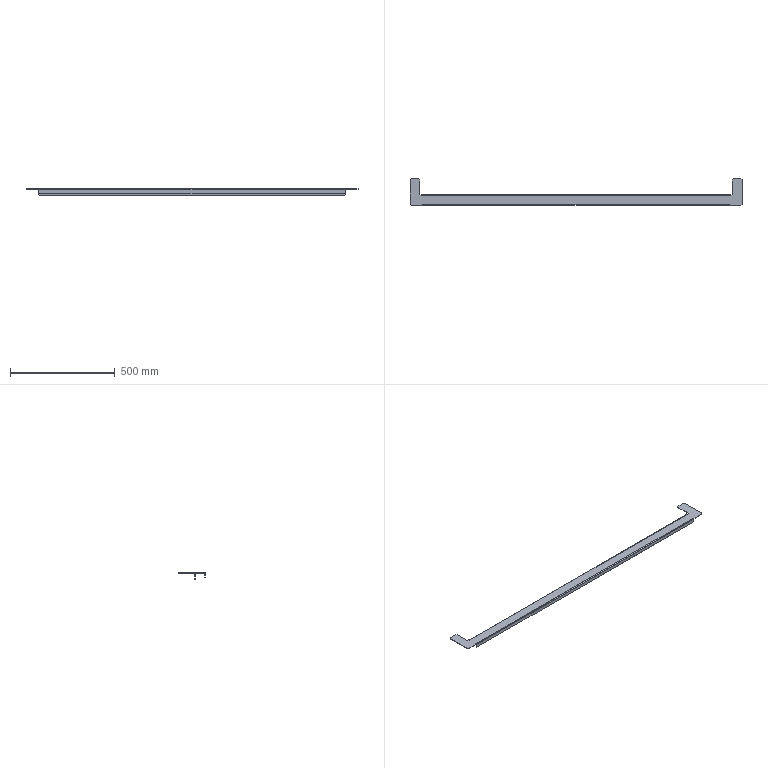Part | STEP file | SYL_0392D6J1SYL0380DJ10-1266534 | 1 solid | 50 faces | box 1586 x 125 x 30 mm | volume 300199 mm3 | plane 46 | cylinder 4 | commonest cylinder face diameters 4 x2 8 x2
STEP:
#1=CARTESIAN_POINT('',(733.,-62.5,-18.));
#2=VERTEX_POINT('',#1);
#3=CARTESIAN_POINT('',(733.,-60.5,-18.));
#4=VERTEX_POINT('',#3);
#5=CARTESIAN_POINT('',(733.,-60.5,-18.));
#6=DIRECTION('',(0.,1.,0.));
#7=VECTOR('',#6,1000.);
#8=LINE('',#5,#7);
#9=EDGE_CURVE('',#2,#4,#8,.T.);
#10=ORIENTED_EDGE('',*,*,#9,.F.);
#11=CARTESIAN_POINT('',(-733.,-62.5,-18.));
#12=VERTEX_POINT('',#11);
#13=CARTESIAN_POINT('',(-793.,-62.5,-18.));
#14=DIRECTION('',(-1.,0.,0.));
#15=VECTOR('',#14,1000.);
#16=LINE('',#13,#15);
#17=EDGE_CURVE('',#2,#12,#16,.T.);
#18=ORIENTED_EDGE('',*,*,#17,.T.);
#19=CARTESIAN_POINT('',(-733.,-60.5,-18.));
#20=VERTEX_POINT('',#19);
#21=CARTESIAN_POINT('',(-733.,-60.5,-18.));
#22=DIRECTION('',(0.,1.,0.));
#23=VECTOR('',#22,1000.);
#24=LINE('',#21,#23);
#25=EDGE_CURVE('',#12,#20,#24,.T.);
#26=ORIENTED_EDGE('',*,*,#25,.T.);
#27=CARTESIAN_POINT('',(733.,-60.5,-18.));
#28=DIRECTION('',(-1.,0.,0.));
#29=VECTOR('',#28,1000.);
#30=LINE('',#27,#29);
#31=EDGE_CURVE('',#4,#20,#30,.T.);
#32=ORIENTED_EDGE('',*,*,#31,.F.);
#33=EDGE_LOOP('',(#10,#18,#26,#32));
#34=FACE_OUTER_BOUND('',#33,.T.);
#35=CARTESIAN_POINT('',(733.,-60.5,-18.));
#36=DIRECTION('',(0.,0.,1.));
#37=DIRECTION('',(-1.,0.,0.));
#38=AXIS2_PLACEMENT_3D('',#35,#36,#37);
#39=PLANE('',#38);
#40=ADVANCED_FACE('',(#34),#39,.F.);
#41=ORIENTED_EDGE('',*,*,#25,.F.);
#42=CARTESIAN_POINT('',(-733.,-62.5,-2.));
#43=VERTEX_POINT('',#42);
#44=CARTESIAN_POINT('',(-733.,-62.5,2.));
#45=DIRECTION('',(0.,0.,1.));
#46=VECTOR('',#45,1000.);
#47=LINE('',#44,#46);
#48=EDGE_CURVE('',#12,#43,#47,.T.);
#49=ORIENTED_EDGE('',*,*,#48,.T.);
#50=CARTESIAN_POINT('',(-733.,-60.5,-2.));
#51=VERTEX_POINT('',#50);
#52=CARTESIAN_POINT('',(-733.,-60.5,-2.));
#53=DIRECTION('',(0.,1.,0.));
#54=VECTOR('',#53,1000.);
#55=LINE('',#52,#54);
#56=EDGE_CURVE('',#43,#51,#55,.T.);
#57=ORIENTED_EDGE('',*,*,#56,.T.);
#58=CARTESIAN_POINT('',(-733.,-60.5,-18.));
#59=DIRECTION('',(0.,0.,1.));
#60=VECTOR('',#59,1000.);
#61=LINE('',#58,#60);
#62=EDGE_CURVE('',#20,#51,#61,.T.);
#63=ORIENTED_EDGE('',*,*,#62,.F.);
#64=EDGE_LOOP('',(#41,#49,#57,#63));
#65=FACE_OUTER_BOUND('',#64,.T.);
#66=CARTESIAN_POINT('',(-733.,-60.5,-18.));
#67=DIRECTION('',(1.,0.,0.));
#68=DIRECTION('',(0.,0.,1.));
#69=AXIS2_PLACEMENT_3D('',#66,#67,#68);
#70=PLANE('',#69);
#71=ADVANCED_FACE('',(#65),#70,.F.);
#72=ORIENTED_EDGE('',*,*,#56,.F.);
#73=CARTESIAN_POINT('',(-733.,-58.5,2.));
#74=VERTEX_POINT('',#73);
#75=CARTESIAN_POINT('',(-733.,-58.5,-2.));
#76=DIRECTION('',(1.,0.,0.));
#77=DIRECTION('',(0.,0.,1.));
#78=AXIS2_PLACEMENT_3D('',#75,#76,#77);
#79=CIRCLE('',#78,4.);
#80=EDGE_CURVE('',#74,#43,#79,.T.);
#81=ORIENTED_EDGE('',*,*,#80,.F.);
#82=CARTESIAN_POINT('',(-733.,-58.5,0.));
#83=VERTEX_POINT('',#82);
#84=CARTESIAN_POINT('',(-733.,-58.5,0.));
#85=DIRECTION('',(0.,0.,-1.));
#86=VECTOR('',#85,1000.);
#87=LINE('',#84,#86);
#88=EDGE_CURVE('',#74,#83,#87,.T.);
#89=ORIENTED_EDGE('',*,*,#88,.T.);
#90=CARTESIAN_POINT('',(-733.,-58.5,-2.));
#91=DIRECTION('',(1.,0.,0.));
#92=DIRECTION('',(0.,0.,1.));
#93=AXIS2_PLACEMENT_3D('',#90,#91,#92);
#94=CIRCLE('',#93,2.);
#95=EDGE_CURVE('',#83,#51,#94,.T.);
#96=ORIENTED_EDGE('',*,*,#95,.T.);
#97=EDGE_LOOP('',(#72,#81,#89,#96));
#98=FACE_OUTER_BOUND('',#97,.T.);
#99=CARTESIAN_POINT('',(-733.,-58.5,-2.));
#100=DIRECTION('',(-1.,0.,0.));
#101=DIRECTION('',(0.,0.,1.));
#102=AXIS2_PLACEMENT_3D('',#99,#100,#101);
#103=PLANE('',#102);
#104=ADVANCED_FACE('',(#98),#103,.T.);
#105=ORIENTED_EDGE('',*,*,#88,.F.);
#106=CARTESIAN_POINT('',(-733.,-57.5,2.));
#107=VERTEX_POINT('',#106);
#108=CARTESIAN_POINT('',(-733.,0.,2.));
#109=DIRECTION('',(0.,1.,0.));
#110=VECTOR('',#109,1000.);
#111=LINE('',#108,#110);
#112=EDGE_CURVE('',#74,#107,#111,.T.);
#113=ORIENTED_EDGE('',*,*,#112,.T.);
#114=CARTESIAN_POINT('',(-733.,-57.5,0.));
#115=VERTEX_POINT('',#114);
#116=CARTESIAN_POINT('',(-733.,-57.5,0.));
#117=DIRECTION('',(0.,0.,-1.));
#118=VECTOR('',#117,1000.);
#119=LINE('',#116,#118);
#120=EDGE_CURVE('',#107,#115,#119,.T.);
#121=ORIENTED_EDGE('',*,*,#120,.T.);
#122=CARTESIAN_POINT('',(-733.,0.,0.));
#123=DIRECTION('',(0.,1.,0.));
#124=VECTOR('',#123,1000.);
#125=LINE('',#122,#124);
#126=EDGE_CURVE('',#83,#115,#125,.T.);
#127=ORIENTED_EDGE('',*,*,#126,.F.);
#128=EDGE_LOOP('',(#105,#113,#121,#127));
#129=FACE_OUTER_BOUND('',#128,.T.);
#130=CARTESIAN_POINT('',(-733.,0.,0.));
#131=DIRECTION('',(1.,0.,0.));
#132=DIRECTION('',(0.,1.,0.));
#133=AXIS2_PLACEMENT_3D('',#130,#131,#132);
#134=PLANE('',#133);
#135=ADVANCED_FACE('',(#129),#134,.F.);
#136=ORIENTED_EDGE('',*,*,#120,.F.);
#137=CARTESIAN_POINT('',(-734.,-57.5,2.));
#138=VERTEX_POINT('',#137);
#139=CARTESIAN_POINT('',(0.,-57.5,2.));
#140=DIRECTION('',(-1.,0.,0.));
#141=VECTOR('',#140,1000.);
#142=LINE('',#139,#141);
#143=EDGE_CURVE('',#107,#138,#142,.T.);
#144=ORIENTED_EDGE('',*,*,#143,.T.);
#145=CARTESIAN_POINT('',(-734.,-57.5,0.));
#146=VERTEX_POINT('',#145);
#147=CARTESIAN_POINT('',(-734.,-57.5,0.));
#148=DIRECTION('',(0.,0.,-1.));
#149=VECTOR('',#148,1000.);
#150=LINE('',#147,#149);
#151=EDGE_CURVE('',#138,#146,#150,.T.);
#152=ORIENTED_EDGE('',*,*,#151,.T.);
#153=CARTESIAN_POINT('',(0.,-57.5,0.));
#154=DIRECTION('',(-1.,0.,0.));
#155=VECTOR('',#154,1000.);
#156=LINE('',#153,#155);
#157=EDGE_CURVE('',#115,#146,#156,.T.);
#158=ORIENTED_EDGE('',*,*,#157,.F.);
#159=EDGE_LOOP('',(#136,#144,#152,#158));
#160=FACE_OUTER_BOUND('',#159,.T.);
#161=CARTESIAN_POINT('',(0.,-57.5,0.));
#162=DIRECTION('',(0.,1.,0.));
#163=DIRECTION('',(-1.,0.,0.));
#164=AXIS2_PLACEMENT_3D('',#161,#162,#163);
#165=PLANE('',#164);
#166=ADVANCED_FACE('',(#160),#165,.F.);
#167=ORIENTED_EDGE('',*,*,#151,.F.);
#168=CARTESIAN_POINT('',(-734.,-62.5,2.));
#169=VERTEX_POINT('',#168);
#170=CARTESIAN_POINT('',(-734.,0.,2.));
#171=DIRECTION('',(0.,-1.,0.));
#172=VECTOR('',#171,1000.);
#173=LINE('',#170,#172);
#174=EDGE_CURVE('',#138,#169,#173,.T.);
#175=ORIENTED_EDGE('',*,*,#174,.T.);
#176=CARTESIAN_POINT('',(-734.,-62.5,0.));
#177=VERTEX_POINT('',#176);
#178=CARTESIAN_POINT('',(-734.,-62.5,0.));
#179=DIRECTION('',(0.,0.,-1.));
#180=VECTOR('',#179,1000.);
#181=LINE('',#178,#180);
#182=EDGE_CURVE('',#169,#177,#181,.T.);
#183=ORIENTED_EDGE('',*,*,#182,.T.);
#184=CARTESIAN_POINT('',(-734.,0.,0.));
#185=DIRECTION('',(0.,-1.,0.));
#186=VECTOR('',#185,1000.);
#187=LINE('',#184,#186);
#188=EDGE_CURVE('',#146,#177,#187,.T.);
#189=ORIENTED_EDGE('',*,*,#188,.F.);
#190=EDGE_LOOP('',(#167,#175,#183,#189));
#191=FACE_OUTER_BOUND('',#190,.T.);
#192=CARTESIAN_POINT('',(-734.,0.,0.));
#193=DIRECTION('',(-1.,0.,0.));
#194=DIRECTION('',(0.,-1.,0.));
#195=AXIS2_PLACEMENT_3D('',#192,#193,#194);
#196=PLANE('',#195);
#197=ADVANCED_FACE('',(#191),#196,.F.);
#198=ORIENTED_EDGE('',*,*,#182,.F.);
#199=CARTESIAN_POINT('',(-788.,-62.5,2.));
#200=VERTEX_POINT('',#199);
#201=CARTESIAN_POINT('',(0.,-62.5,2.));
#202=DIRECTION('',(-1.,0.,0.));
#203=VECTOR('',#202,1000.);
#204=LINE('',#201,#203);
#205=EDGE_CURVE('',#169,#200,#204,.T.);
#206=ORIENTED_EDGE('',*,*,#205,.T.);
#207=CARTESIAN_POINT('',(-788.,-62.5,0.));
#208=VERTEX_POINT('',#207);
#209=CARTESIAN_POINT('',(-788.,-62.5,0.));
#210=DIRECTION('',(0.,0.,-1.));
#211=VECTOR('',#210,1000.);
#212=LINE('',#209,#211);
#213=EDGE_CURVE('',#200,#208,#212,.T.);
#214=ORIENTED_EDGE('',*,*,#213,.T.);
#215=CARTESIAN_POINT('',(-733.,-62.5,0.));
#216=DIRECTION('',(-1.,0.,0.));
#217=VECTOR('',#216,1000.);
#218=LINE('',#215,#217);
#219=EDGE_CURVE('',#177,#208,#218,.T.);
#220=ORIENTED_EDGE('',*,*,#219,.F.);
#221=EDGE_LOOP('',(#198,#206,#214,#220));
#222=FACE_OUTER_BOUND('',#221,.T.);
#223=CARTESIAN_POINT('',(-733.,-62.5,0.));
#224=DIRECTION('',(0.,1.,0.));
#225=DIRECTION('',(-1.,0.,0.));
#226=AXIS2_PLACEMENT_3D('',#223,#224,#225);
#227=PLANE('',#226);
#228=ADVANCED_FACE('',(#222),#227,.F.);
#229=ORIENTED_EDGE('',*,*,#213,.F.);
#230=CARTESIAN_POINT('',(-793.,-57.5,2.));
#231=VERTEX_POINT('',#230);
#232=CARTESIAN_POINT('',(-788.,-62.5,2.));
#233=DIRECTION('',(-0.7071,0.7071,0.));
#234=VECTOR('',#233,1000.);
#235=LINE('',#232,#234);
#236=EDGE_CURVE('',#200,#231,#235,.T.);
#237=ORIENTED_EDGE('',*,*,#236,.T.);
#238=CARTESIAN_POINT('',(-793.,-57.5,0.));
#239=VERTEX_POINT('',#238);
#240=CARTESIAN_POINT('',(-793.,-57.5,0.));
#241=DIRECTION('',(0.,0.,-1.));
#242=VECTOR('',#241,1000.);
#243=LINE('',#240,#242);
#244=EDGE_CURVE('',#231,#239,#243,.T.);
#245=ORIENTED_EDGE('',*,*,#244,.T.);
#246=CARTESIAN_POINT('',(-788.,-62.5,0.));
#247=DIRECTION('',(-0.7071,0.7071,0.));
#248=VECTOR('',#247,1000.);
#249=LINE('',#246,#248);
#250=EDGE_CURVE('',#208,#239,#249,.T.);
#251=ORIENTED_EDGE('',*,*,#250,.F.);
#252=EDGE_LOOP('',(#229,#237,#245,#251));
#253=FACE_OUTER_BOUND('',#252,.T.);
#254=CARTESIAN_POINT('',(-788.,-62.5,0.));
#255=DIRECTION('',(0.7071,0.7071,0.));
#256=DIRECTION('',(-0.7071,0.7071,0.));
#257=AXIS2_PLACEMENT_3D('',#254,#255,#256);
#258=PLANE('',#257);
#259=ADVANCED_FACE('',(#253),#258,.F.);
#260=ORIENTED_EDGE('',*,*,#244,.F.);
#261=CARTESIAN_POINT('',(-793.,57.5,2.));
#262=VERTEX_POINT('',#261);
#263=CARTESIAN_POINT('',(-793.,0.,2.));
#264=DIRECTION('',(0.,1.,0.));
#265=VECTOR('',#264,1000.);
#266=LINE('',#263,#265);
#267=EDGE_CURVE('',#231,#262,#266,.T.);
#268=ORIENTED_EDGE('',*,*,#267,.T.);
#269=CARTESIAN_POINT('',(-793.,57.5,0.));
#270=VERTEX_POINT('',#269);
#271=CARTESIAN_POINT('',(-793.,57.5,0.));
#272=DIRECTION('',(0.,0.,-1.));
#273=VECTOR('',#272,1000.);
#274=LINE('',#271,#273);
#275=EDGE_CURVE('',#262,#270,#274,.T.);
#276=ORIENTED_EDGE('',*,*,#275,.T.);
#277=CARTESIAN_POINT('',(-793.,-57.5,0.));
#278=DIRECTION('',(0.,1.,0.));
#279=VECTOR('',#278,1000.);
#280=LINE('',#277,#279);
#281=EDGE_CURVE('',#239,#270,#280,.T.);
#282=ORIENTED_EDGE('',*,*,#281,.F.);
#283=EDGE_LOOP('',(#260,#268,#276,#282));
#284=FACE_OUTER_BOUND('',#283,.T.);
#285=CARTESIAN_POINT('',(-793.,-57.5,0.));
#286=DIRECTION('',(1.,0.,0.));
#287=DIRECTION('',(0.,1.,0.));
#288=AXIS2_PLACEMENT_3D('',#285,#286,#287);
#289=PLANE('',#288);
#290=ADVANCED_FACE('',(#284),#289,.F.);
#291=ORIENTED_EDGE('',*,*,#275,.F.);
#292=CARTESIAN_POINT('',(-788.,62.5,2.));
#293=VERTEX_POINT('',#292);
#294=CARTESIAN_POINT('',(-793.,57.5,2.));
#295=DIRECTION('',(0.7071,0.7071,0.));
#296=VECTOR('',#295,1000.);
#297=LINE('',#294,#296);
#298=EDGE_CURVE('',#262,#293,#297,.T.);
#299=ORIENTED_EDGE('',*,*,#298,.T.);
#300=CARTESIAN_POINT('',(-788.,62.5,0.));
#301=VERTEX_POINT('',#300);
#302=CARTESIAN_POINT('',(-788.,62.5,0.));
#303=DIRECTION('',(0.,0.,-1.));
#304=VECTOR('',#303,1000.);
#305=LINE('',#302,#304);
#306=EDGE_CURVE('',#293,#301,#305,.T.);
#307=ORIENTED_EDGE('',*,*,#306,.T.);
#308=CARTESIAN_POINT('',(-793.,57.5,0.));
#309=DIRECTION('',(0.7071,0.7071,0.));
#310=VECTOR('',#309,1000.);
#311=LINE('',#308,#310);
#312=EDGE_CURVE('',#270,#301,#311,.T.);
#313=ORIENTED_EDGE('',*,*,#312,.F.);
#314=EDGE_LOOP('',(#291,#299,#307,#313));
#315=FACE_OUTER_BOUND('',#314,.T.);
#316=CARTESIAN_POINT('',(-793.,57.5,0.));
#317=DIRECTION('',(0.7071,-0.7071,0.));
#318=DIRECTION('',(0.7071,0.7071,0.));
#319=AXIS2_PLACEMENT_3D('',#316,#317,#318);
#320=PLANE('',#319);
#321=ADVANCED_FACE('',(#315),#320,.F.);
#322=ORIENTED_EDGE('',*,*,#306,.F.);
#323=CARTESIAN_POINT('',(-750.5,62.5,2.));
#324=VERTEX_POINT('',#323);
#325=CARTESIAN_POINT('',(0.,62.5,2.));
#326=DIRECTION('',(1.,0.,0.));
#327=VECTOR('',#326,1000.);
#328=LINE('',#325,#327);
#329=EDGE_CURVE('',#293,#324,#328,.T.);
#330=ORIENTED_EDGE('',*,*,#329,.T.);
#331=CARTESIAN_POINT('',(-750.5,62.5,0.));
#332=VERTEX_POINT('',#331);
#333=CARTESIAN_POINT('',(-750.5,62.5,0.));
#334=DIRECTION('',(0.,0.,-1.));
#335=VECTOR('',#334,1000.);
#336=LINE('',#333,#335);
#337=EDGE_CURVE('',#324,#332,#336,.T.);
#338=ORIENTED_EDGE('',*,*,#337,.T.);
#339=CARTESIAN_POINT('',(-788.,62.5,0.));
#340=DIRECTION('',(1.,0.,0.));
#341=VECTOR('',#340,1000.);
#342=LINE('',#339,#341);
#343=EDGE_CURVE('',#301,#332,#342,.T.);
#344=ORIENTED_EDGE('',*,*,#343,.F.);
#345=EDGE_LOOP('',(#322,#330,#338,#344));
#346=FACE_OUTER_BOUND('',#345,.T.);
#347=CARTESIAN_POINT('',(-788.,62.5,0.));
#348=DIRECTION('',(0.,-1.,0.));
#349=DIRECTION('',(1.,0.,0.));
#350=AXIS2_PLACEMENT_3D('',#347,#348,#349);
#351=PLANE('',#350);
#352=ADVANCED_FACE('',(#346),#351,.F.);
#353=ORIENTED_EDGE('',*,*,#337,.F.);
#354=CARTESIAN_POINT('',(-745.5,57.5,2.));
#355=VERTEX_POINT('',#354);
#356=CARTESIAN_POINT('',(-750.5,62.5,2.));
#357=DIRECTION('',(0.7071,-0.7071,0.));
#358=VECTOR('',#357,1000.);
#359=LINE('',#356,#358);
#360=EDGE_CURVE('',#324,#355,#359,.T.);
#361=ORIENTED_EDGE('',*,*,#360,.T.);
#362=CARTESIAN_POINT('',(-745.5,57.5,0.));
#363=VERTEX_POINT('',#362);
#364=CARTESIAN_POINT('',(-745.5,57.5,0.));
#365=DIRECTION('',(0.,0.,-1.));
#366=VECTOR('',#365,1000.);
#367=LINE('',#364,#366);
#368=EDGE_CURVE('',#355,#363,#367,.T.);
#369=ORIENTED_EDGE('',*,*,#368,.T.);
#370=CARTESIAN_POINT('',(-750.5,62.5,0.));
#371=DIRECTION('',(0.7071,-0.7071,0.));
#372=VECTOR('',#371,1000.);
#373=LINE('',#370,#372);
#374=EDGE_CURVE('',#332,#363,#373,.T.);
#375=ORIENTED_EDGE('',*,*,#374,.F.);
#376=EDGE_LOOP('',(#353,#361,#369,#375));
#377=FACE_OUTER_BOUND('',#376,.T.);
#378=CARTESIAN_POINT('',(-750.5,62.5,0.));
#379=DIRECTION('',(-0.7071,-0.7071,0.));
#380=DIRECTION('',(0.7071,-0.7071,0.));
#381=AXIS2_PLACEMENT_3D('',#378,#379,#380);
#382=PLANE('',#381);
#383=ADVANCED_FACE('',(#377),#382,.F.);
#384=ORIENTED_EDGE('',*,*,#368,.F.);
#385=CARTESIAN_POINT('',(-745.5,-12.5,2.));
#386=VERTEX_POINT('',#385);
#387=CARTESIAN_POINT('',(-745.5,0.,2.));
#388=DIRECTION('',(0.,-1.,0.));
#389=VECTOR('',#388,1000.);
#390=LINE('',#387,#389);
#391=EDGE_CURVE('',#355,#386,#390,.T.);
#392=ORIENTED_EDGE('',*,*,#391,.T.);
#393=CARTESIAN_POINT('',(-745.5,-12.5,0.));
#394=VERTEX_POINT('',#393);
#395=CARTESIAN_POINT('',(-745.5,-12.5,0.));
#396=DIRECTION('',(0.,0.,-1.));
#397=VECTOR('',#396,1000.);
#398=LINE('',#395,#397);
#399=EDGE_CURVE('',#386,#394,#398,.T.);
#400=ORIENTED_EDGE('',*,*,#399,.T.);
#401=CARTESIAN_POINT('',(-745.5,57.5,0.));
#402=DIRECTION('',(0.,-1.,0.));
#403=VECTOR('',#402,1000.);
#404=LINE('',#401,#403);
#405=EDGE_CURVE('',#363,#394,#404,.T.);
#406=ORIENTED_EDGE('',*,*,#405,.F.);
#407=EDGE_LOOP('',(#384,#392,#400,#406));
#408=FACE_OUTER_BOUND('',#407,.T.);
#409=CARTESIAN_POINT('',(-745.5,57.5,0.));
#410=DIRECTION('',(-1.,0.,0.));
#411=DIRECTION('',(0.,-1.,0.));
#412=AXIS2_PLACEMENT_3D('',#409,#410,#411);
#413=PLANE('',#412);
#414=ADVANCED_FACE('',(#408),#413,.F.);
#415=ORIENTED_EDGE('',*,*,#399,.F.);
#416=CARTESIAN_POINT('',(-736.5,-12.5,2.));
#417=VERTEX_POINT('',#416);
#418=CARTESIAN_POINT('',(0.,-12.5,2.));
#419=DIRECTION('',(1.,0.,0.));
#420=VECTOR('',#419,1000.);
#421=LINE('',#418,#420);
#422=EDGE_CURVE('',#386,#417,#421,.T.);
#423=ORIENTED_EDGE('',*,*,#422,.T.);
#424=CARTESIAN_POINT('',(-736.5,-12.5,0.));
#425=VERTEX_POINT('',#424);
#426=CARTESIAN_POINT('',(-736.5,-12.5,0.));
#427=DIRECTION('',(0.,0.,-1.));
#428=VECTOR('',#427,1000.);
#429=LINE('',#426,#428);
#430=EDGE_CURVE('',#417,#425,#429,.T.);
#431=ORIENTED_EDGE('',*,*,#430,.T.);
#432=CARTESIAN_POINT('',(-745.5,-12.5,0.));
#433=DIRECTION('',(1.,0.,0.));
#434=VECTOR('',#433,1000.);
#435=LINE('',#432,#434);
#436=EDGE_CURVE('',#394,#425,#435,.T.);
#437=ORIENTED_EDGE('',*,*,#436,.F.);
#438=EDGE_LOOP('',(#415,#423,#431,#437));
#439=FACE_OUTER_BOUND('',#438,.T.);
#440=CARTESIAN_POINT('',(-745.5,-12.5,0.));
#441=DIRECTION('',(0.,-1.,0.));
#442=DIRECTION('',(1.,0.,0.));
#443=AXIS2_PLACEMENT_3D('',#440,#441,#442);
#444=PLANE('',#443);
#445=ADVANCED_FACE('',(#439),#444,.F.);
#446=ORIENTED_EDGE('',*,*,#430,.F.);
#447=CARTESIAN_POINT('',(-736.5,-17.5,2.));
#448=VERTEX_POINT('',#447);
#449=CARTESIAN_POINT('',(-736.5,0.,2.));
#450=DIRECTION('',(0.,-1.,0.));
#451=VECTOR('',#450,1000.);
#452=LINE('',#449,#451);
#453=EDGE_CURVE('',#417,#448,#452,.T.);
#454=ORIENTED_EDGE('',*,*,#453,.T.);
#455=CARTESIAN_POINT('',(-736.5,-17.5,0.));
#456=VERTEX_POINT('',#455);
#457=CARTESIAN_POINT('',(-736.5,-17.5,0.));
#458=DIRECTION('',(0.,0.,-1.));
#459=VECTOR('',#458,1000.);
#460=LINE('',#457,#459);
#461=EDGE_CURVE('',#448,#456,#460,.T.);
#462=ORIENTED_EDGE('',*,*,#461,.T.);
#463=CARTESIAN_POINT('',(-736.5,0.,0.));
#464=DIRECTION('',(0.,-1.,0.));
#465=VECTOR('',#464,1000.);
#466=LINE('',#463,#465);
#467=EDGE_CURVE('',#425,#456,#466,.T.);
#468=ORIENTED_EDGE('',*,*,#467,.F.);
#469=EDGE_LOOP('',(#446,#454,#462,#468));
#470=FACE_OUTER_BOUND('',#469,.T.);
#471=CARTESIAN_POINT('',(-736.5,0.,0.));
#472=DIRECTION('',(-1.,0.,0.));
#473=DIRECTION('',(0.,-1.,0.));
#474=AXIS2_PLACEMENT_3D('',#471,#472,#473);
#475=PLANE('',#474);
#476=ADVANCED_FACE('',(#470),#475,.F.);
#477=ORIENTED_EDGE('',*,*,#461,.F.);
#478=CARTESIAN_POINT('',(-735.5,-17.5,2.));
#479=VERTEX_POINT('',#478);
#480=CARTESIAN_POINT('',(0.,-17.5,2.));
#481=DIRECTION('',(1.,0.,0.));
#482=VECTOR('',#481,1000.);
#483=LINE('',#480,#482);
#484=EDGE_CURVE('',#448,#479,#483,.T.);
#485=ORIENTED_EDGE('',*,*,#484,.T.);
#486=CARTESIAN_POINT('',(-735.5,-17.5,0.));
#487=VERTEX_POINT('',#486);
#488=CARTESIAN_POINT('',(-735.5,-17.5,0.));
#489=DIRECTION('',(0.,0.,-1.));
#490=VECTOR('',#489,1000.);
#491=LINE('',#488,#490);
#492=EDGE_CURVE('',#479,#487,#491,.T.);
#493=ORIENTED_EDGE('',*,*,#492,.T.);
#494=CARTESIAN_POINT('',(0.,-17.5,0.));
#495=DIRECTION('',(1.,0.,0.));
#496=VECTOR('',#495,1000.);
#497=LINE('',#494,#496);
#498=EDGE_CURVE('',#456,#487,#497,.T.);
#499=ORIENTED_EDGE('',*,*,#498,.F.);
#500=EDGE_LOOP('',(#477,#485,#493,#499));
#501=FACE_OUTER_BOUND('',#500,.T.);
#502=CARTESIAN_POINT('',(0.,-17.5,0.));
#503=DIRECTION('',(0.,-1.,0.));
#504=DIRECTION('',(1.,0.,0.));
#505=AXIS2_PLACEMENT_3D('',#502,#503,#504);
#506=PLANE('',#505);
#507=ADVANCED_FACE('',(#501),#506,.F.);
#508=ORIENTED_EDGE('',*,*,#492,.F.);
#509=CARTESIAN_POINT('',(-735.5,-16.5,2.));
#510=VERTEX_POINT('',#509);
#511=CARTESIAN_POINT('',(-735.5,0.,2.));
#512=DIRECTION('',(0.,1.,0.));
#513=VECTOR('',#512,1000.);
#514=LINE('',#511,#513);
#515=EDGE_CURVE('',#479,#510,#514,.T.);
#516=ORIENTED_EDGE('',*,*,#515,.T.);
#517=CARTESIAN_POINT('',(-735.5,-16.5,0.));
#518=VERTEX_POINT('',#517);
#519=CARTESIAN_POINT('',(-735.5,-16.5,0.));
#520=DIRECTION('',(0.,0.,-1.));
#521=VECTOR('',#520,1000.);
#522=LINE('',#519,#521);
#523=EDGE_CURVE('',#510,#518,#522,.T.);
#524=ORIENTED_EDGE('',*,*,#523,.T.);
#525=CARTESIAN_POINT('',(-735.5,0.,0.));
#526=DIRECTION('',(0.,1.,0.));
#527=VECTOR('',#526,1000.);
#528=LINE('',#525,#527);
#529=EDGE_CURVE('',#487,#518,#528,.T.);
#530=ORIENTED_EDGE('',*,*,#529,.F.);
#531=EDGE_LOOP('',(#508,#516,#524,#530));
#532=FACE_OUTER_BOUND('',#531,.T.);
#533=CARTESIAN_POINT('',(-735.5,0.,0.));
#534=DIRECTION('',(1.,0.,0.));
#535=DIRECTION('',(0.,1.,0.));
#536=AXIS2_PLACEMENT_3D('',#533,#534,#535);
#537=PLANE('',#536);
#538=ADVANCED_FACE('',(#532),#537,.F.);
#539=ORIENTED_EDGE('',*,*,#523,.F.);
#540=CARTESIAN_POINT('',(-735.5,-12.5,-2.));
#541=VERTEX_POINT('',#540);
#542=CARTESIAN_POINT('',(-735.5,-16.5,-2.));
#543=DIRECTION('',(1.,0.,0.));
#544=DIRECTION('',(0.,0.,-1.));
#545=AXIS2_PLACEMENT_3D('',#542,#543,#544);
#546=CIRCLE('',#545,4.);
#547=EDGE_CURVE('',#541,#510,#546,.T.);
#548=ORIENTED_EDGE('',*,*,#547,.F.);
#549=CARTESIAN_POINT('',(-735.5,-14.5,-2.));
#550=VERTEX_POINT('',#549);
#551=CARTESIAN_POINT('',(-735.5,-14.5,-2.));
#552=DIRECTION('',(0.,-1.,0.));
#553=VECTOR('',#552,1000.);
#554=LINE('',#551,#553);
#555=EDGE_CURVE('',#541,#550,#554,.T.);
#556=ORIENTED_EDGE('',*,*,#555,.T.);
#557=CARTESIAN_POINT('',(-735.5,-16.5,-2.));
#558=DIRECTION('',(1.,0.,0.));
#559=DIRECTION('',(0.,1.,0.));
#560=AXIS2_PLACEMENT_3D('',#557,#558,#559);
#561=CIRCLE('',#560,2.);
#562=EDGE_CURVE('',#550,#518,#561,.T.);
#563=ORIENTED_EDGE('',*,*,#562,.T.);
#564=EDGE_LOOP('',(#539,#548,#556,#563));
#565=FACE_OUTER_BOUND('',#564,.T.);
#566=CARTESIAN_POINT('',(-735.5,-16.5,-2.));
#567=DIRECTION('',(-1.,0.,0.));
#568=DIRECTION('',(0.,0.,1.));
#569=AXIS2_PLACEMENT_3D('',#566,#567,#568);
#570=PLANE('',#569);
#571=ADVANCED_FACE('',(#565),#570,.T.);
#572=ORIENTED_EDGE('',*,*,#555,.F.);
#573=CARTESIAN_POINT('',(-735.5,-12.5,-23.));
#574=VERTEX_POINT('',#573);
#575=CARTESIAN_POINT('',(-735.5,-12.5,2.));
#576=DIRECTION('',(0.,0.,-1.));
#577=VECTOR('',#576,1000.);
#578=LINE('',#575,#577);
#579=EDGE_CURVE('',#541,#574,#578,.T.);
#580=ORIENTED_EDGE('',*,*,#579,.T.);
#581=CARTESIAN_POINT('',(-735.5,-14.5,-23.));
#582=VERTEX_POINT('',#581);
#583=CARTESIAN_POINT('',(-735.5,-14.5,-23.));
#584=DIRECTION('',(0.,-1.,0.));
#585=VECTOR('',#584,1000.);
#586=LINE('',#583,#585);
#587=EDGE_CURVE('',#574,#582,#586,.T.);
#588=ORIENTED_EDGE('',*,*,#587,.T.);
#589=CARTESIAN_POINT('',(-735.5,-14.5,-2.));
#590=DIRECTION('',(0.,0.,-1.));
#591=VECTOR('',#590,1000.);
#592=LINE('',#589,#591);
#593=EDGE_CURVE('',#550,#582,#592,.T.);
#594=ORIENTED_EDGE('',*,*,#593,.F.);
#595=EDGE_LOOP('',(#572,#580,#588,#594));
#596=FACE_OUTER_BOUND('',#595,.T.);
#597=CARTESIAN_POINT('',(-735.5,-14.5,-2.));
#598=DIRECTION('',(1.,0.,0.));
#599=DIRECTION('',(0.,0.,-1.));
#600=AXIS2_PLACEMENT_3D('',#597,#598,#599);
#601=PLANE('',#600);
#602=ADVANCED_FACE('',(#596),#601,.F.);
#603=ORIENTED_EDGE('',*,*,#587,.F.);
#604=CARTESIAN_POINT('',(-730.5,-12.5,-28.));
#605=VERTEX_POINT('',#604);
#606=CARTESIAN_POINT('',(-735.5,-12.5,-23.));
#607=DIRECTION('',(0.7071,0.,-0.7071));
#608=VECTOR('',#607,1000.);
#609=LINE('',#606,#608);
#610=EDGE_CURVE('',#574,#605,#609,.T.);
#611=ORIENTED_EDGE('',*,*,#610,.T.);
#612=CARTESIAN_POINT('',(-730.5,-14.5,-28.));
#613=VERTEX_POINT('',#612);
#614=CARTESIAN_POINT('',(-730.5,-14.5,-28.));
#615=DIRECTION('',(0.,-1.,0.));
#616=VECTOR('',#615,1000.);
#617=LINE('',#614,#616);
#618=EDGE_CURVE('',#605,#613,#617,.T.);
#619=ORIENTED_EDGE('',*,*,#618,.T.);
#620=CARTESIAN_POINT('',(-735.5,-14.5,-23.));
#621=DIRECTION('',(0.7071,0.,-0.7071));
#622=VECTOR('',#621,1000.);
#623=LINE('',#620,#622);
#624=EDGE_CURVE('',#582,#613,#623,.T.);
#625=ORIENTED_EDGE('',*,*,#624,.F.);
#626=EDGE_LOOP('',(#603,#611,#619,#625));
#627=FACE_OUTER_BOUND('',#626,.T.);
#628=CARTESIAN_POINT('',(-735.5,-14.5,-23.));
#629=DIRECTION('',(0.7071,0.,0.7071));
#630=DIRECTION('',(0.7071,0.,-0.7071));
#631=AXIS2_PLACEMENT_3D('',#628,#629,#630);
#632=PLANE('',#631);
#633=ADVANCED_FACE('',(#627),#632,.F.);
#634=ORIENTED_EDGE('',*,*,#618,.F.);
#635=CARTESIAN_POINT('',(730.5,-12.5,-28.));
#636=VERTEX_POINT('',#635);
#637=CARTESIAN_POINT('',(745.5,-12.5,-28.));
#638=DIRECTION('',(1.,0.,0.));
#639=VECTOR('',#638,1000.);
#640=LINE('',#637,#639);
#641=EDGE_CURVE('',#605,#636,#640,.T.);
#642=ORIENTED_EDGE('',*,*,#641,.T.);
#643=CARTESIAN_POINT('',(730.5,-14.5,-28.));
#644=VERTEX_POINT('',#643);
#645=CARTESIAN_POINT('',(730.5,-14.5,-28.));
#646=DIRECTION('',(0.,-1.,0.));
#647=VECTOR('',#646,1000.);
#648=LINE('',#645,#647);
#649=EDGE_CURVE('',#636,#644,#648,.T.);
#650=ORIENTED_EDGE('',*,*,#649,.T.);
#651=CARTESIAN_POINT('',(-730.5,-14.5,-28.));
#652=DIRECTION('',(1.,0.,0.));
#653=VECTOR('',#652,1000.);
#654=LINE('',#651,#653);
#655=EDGE_CURVE('',#613,#644,#654,.T.);
#656=ORIENTED_EDGE('',*,*,#655,.F.);
#657=EDGE_LOOP('',(#634,#642,#650,#656));
#658=FACE_OUTER_BOUND('',#657,.T.);
#659=CARTESIAN_POINT('',(-730.5,-14.5,-28.));
#660=DIRECTION('',(0.,0.,1.));
#661=DIRECTION('',(1.,0.,0.));
#662=AXIS2_PLACEMENT_3D('',#659,#660,#661);
#663=PLANE('',#662);
#664=ADVANCED_FACE('',(#658),#663,.F.);
#665=ORIENTED_EDGE('',*,*,#649,.F.);
#666=CARTESIAN_POINT('',(735.5,-12.5,-23.));
#667=VERTEX_POINT('',#666);
#668=CARTESIAN_POINT('',(730.5,-12.5,-28.));
#669=DIRECTION('',(0.7071,0.,0.7071));
#670=VECTOR('',#669,1000.);
#671=LINE('',#668,#670);
#672=EDGE_CURVE('',#636,#667,#671,.T.);
#673=ORIENTED_EDGE('',*,*,#672,.T.);
#674=CARTESIAN_POINT('',(735.5,-14.5,-23.));
#675=VERTEX_POINT('',#674);
#676=CARTESIAN_POINT('',(735.5,-14.5,-23.));
#677=DIRECTION('',(0.,-1.,0.));
#678=VECTOR('',#677,1000.);
#679=LINE('',#676,#678);
#680=EDGE_CURVE('',#667,#675,#679,.T.);
#681=ORIENTED_EDGE('',*,*,#680,.T.);
#682=CARTESIAN_POINT('',(730.5,-14.5,-28.));
#683=DIRECTION('',(0.7071,0.,0.7071));
#684=VECTOR('',#683,1000.);
#685=LINE('',#682,#684);
#686=EDGE_CURVE('',#644,#675,#685,.T.);
#687=ORIENTED_EDGE('',*,*,#686,.F.);
#688=EDGE_LOOP('',(#665,#673,#681,#687));
#689=FACE_OUTER_BOUND('',#688,.T.);
#690=CARTESIAN_POINT('',(730.5,-14.5,-28.));
#691=DIRECTION('',(-0.7071,0.,0.7071));
#692=DIRECTION('',(0.7071,0.,0.7071));
#693=AXIS2_PLACEMENT_3D('',#690,#691,#692);
#694=PLANE('',#693);
#695=ADVANCED_FACE('',(#689),#694,.F.);
#696=ORIENTED_EDGE('',*,*,#680,.F.);
#697=CARTESIAN_POINT('',(735.5,-12.5,-2.));
#698=VERTEX_POINT('',#697);
#699=CARTESIAN_POINT('',(735.5,-12.5,2.));
#700=DIRECTION('',(0.,0.,1.));
#701=VECTOR('',#700,1000.);
#702=LINE('',#699,#701);
#703=EDGE_CURVE('',#667,#698,#702,.T.);
#704=ORIENTED_EDGE('',*,*,#703,.T.);
#705=CARTESIAN_POINT('',(735.5,-14.5,-2.));
#706=VERTEX_POINT('',#705);
#707=CARTESIAN_POINT('',(735.5,-14.5,-2.));
#708=DIRECTION('',(0.,-1.,0.));
#709=VECTOR('',#708,1000.);
#710=LINE('',#707,#709);
#711=EDGE_CURVE('',#698,#706,#710,.T.);
#712=ORIENTED_EDGE('',*,*,#711,.T.);
#713=CARTESIAN_POINT('',(735.5,-14.5,-23.));
#714=DIRECTION('',(0.,0.,1.));
#715=VECTOR('',#714,1000.);
#716=LINE('',#713,#715);
#717=EDGE_CURVE('',#675,#706,#716,.T.);
#718=ORIENTED_EDGE('',*,*,#717,.F.);
#719=EDGE_LOOP('',(#696,#704,#712,#718));
#720=FACE_OUTER_BOUND('',#719,.T.);
#721=CARTESIAN_POINT('',(735.5,-14.5,-23.));
#722=DIRECTION('',(-1.,0.,0.));
#723=DIRECTION('',(0.,0.,1.));
#724=AXIS2_PLACEMENT_3D('',#721,#722,#723);
#725=PLANE('',#724);
#726=ADVANCED_FACE('',(#720),#725,.F.);
#727=ORIENTED_EDGE('',*,*,#711,.F.);
#728=CARTESIAN_POINT('',(735.5,-16.5,2.));
#729=VERTEX_POINT('',#728);
#730=CARTESIAN_POINT('',(735.5,-16.5,-2.));
#731=DIRECTION('',(-1.,0.,0.));
#732=DIRECTION('',(0.,0.,-1.));
#733=AXIS2_PLACEMENT_3D('',#730,#731,#732);
#734=CIRCLE('',#733,4.);
#735=EDGE_CURVE('',#729,#698,#734,.T.);
#736=ORIENTED_EDGE('',*,*,#735,.F.);
#737=CARTESIAN_POINT('',(735.5,-16.5,0.));
#738=VERTEX_POINT('',#737);
#739=CARTESIAN_POINT('',(735.5,-16.5,0.));
#740=DIRECTION('',(0.,0.,-1.));
#741=VECTOR('',#740,1000.);
#742=LINE('',#739,#741);
#743=EDGE_CURVE('',#729,#738,#742,.T.);
#744=ORIENTED_EDGE('',*,*,#743,.T.);
#745=CARTESIAN_POINT('',(735.5,-16.5,-2.));
#746=DIRECTION('',(-1.,0.,0.));
#747=DIRECTION('',(0.,0.,1.));
#748=AXIS2_PLACEMENT_3D('',#745,#746,#747);
#749=CIRCLE('',#748,2.);
#750=EDGE_CURVE('',#738,#706,#749,.T.);
#751=ORIENTED_EDGE('',*,*,#750,.T.);
#752=EDGE_LOOP('',(#727,#736,#744,#751));
#753=FACE_OUTER_BOUND('',#752,.T.);
#754=CARTESIAN_POINT('',(735.5,-16.5,-2.));
#755=DIRECTION('',(1.,0.,0.));
#756=DIRECTION('',(0.,0.,-1.));
#757=AXIS2_PLACEMENT_3D('',#754,#755,#756);
#758=PLANE('',#757);
#759=ADVANCED_FACE('',(#753),#758,.T.);
#760=ORIENTED_EDGE('',*,*,#743,.F.);
#761=CARTESIAN_POINT('',(735.5,-17.5,2.));
#762=VERTEX_POINT('',#761);
#763=CARTESIAN_POINT('',(735.5,0.,2.));
#764=DIRECTION('',(0.,-1.,0.));
#765=VECTOR('',#764,1000.);
#766=LINE('',#763,#765);
#767=EDGE_CURVE('',#729,#762,#766,.T.);
#768=ORIENTED_EDGE('',*,*,#767,.T.);
#769=CARTESIAN_POINT('',(735.5,-17.5,0.));
#770=VERTEX_POINT('',#769);
#771=CARTESIAN_POINT('',(735.5,-17.5,0.));
#772=DIRECTION('',(0.,0.,-1.));
#773=VECTOR('',#772,1000.);
#774=LINE('',#771,#773);
#775=EDGE_CURVE('',#762,#770,#774,.T.);
#776=ORIENTED_EDGE('',*,*,#775,.T.);
#777=CARTESIAN_POINT('',(735.5,0.,0.));
#778=DIRECTION('',(0.,-1.,0.));
#779=VECTOR('',#778,1000.);
#780=LINE('',#777,#779);
#781=EDGE_CURVE('',#738,#770,#780,.T.);
#782=ORIENTED_EDGE('',*,*,#781,.F.);
#783=EDGE_LOOP('',(#760,#768,#776,#782));
#784=FACE_OUTER_BOUND('',#783,.T.);
#785=CARTESIAN_POINT('',(735.5,0.,0.));
#786=DIRECTION('',(-1.,0.,0.));
#787=DIRECTION('',(0.,-1.,0.));
#788=AXIS2_PLACEMENT_3D('',#785,#786,#787);
#789=PLANE('',#788);
#790=ADVANCED_FACE('',(#784),#789,.F.);
#791=ORIENTED_EDGE('',*,*,#775,.F.);
#792=CARTESIAN_POINT('',(736.5,-17.5,2.));
#793=VERTEX_POINT('',#792);
#794=CARTESIAN_POINT('',(0.,-17.5,2.));
#795=DIRECTION('',(1.,0.,0.));
#796=VECTOR('',#795,1000.);
#797=LINE('',#794,#796);
#798=EDGE_CURVE('',#762,#793,#797,.T.);
#799=ORIENTED_EDGE('',*,*,#798,.T.);
#800=CARTESIAN_POINT('',(736.5,-17.5,0.));
#801=VERTEX_POINT('',#800);
#802=CARTESIAN_POINT('',(736.5,-17.5,0.));
#803=DIRECTION('',(0.,0.,-1.));
#804=VECTOR('',#803,1000.);
#805=LINE('',#802,#804);
#806=EDGE_CURVE('',#793,#801,#805,.T.);
#807=ORIENTED_EDGE('',*,*,#806,.T.);
#808=CARTESIAN_POINT('',(0.,-17.5,0.));
#809=DIRECTION('',(1.,0.,0.));
#810=VECTOR('',#809,1000.);
#811=LINE('',#808,#810);
#812=EDGE_CURVE('',#770,#801,#811,.T.);
#813=ORIENTED_EDGE('',*,*,#812,.F.);
#814=EDGE_LOOP('',(#791,#799,#807,#813));
#815=FACE_OUTER_BOUND('',#814,.T.);
#816=CARTESIAN_POINT('',(0.,-17.5,0.));
#817=DIRECTION('',(0.,-1.,0.));
#818=DIRECTION('',(1.,0.,0.));
#819=AXIS2_PLACEMENT_3D('',#816,#817,#818);
#820=PLANE('',#819);
#821=ADVANCED_FACE('',(#815),#820,.F.);
#822=ORIENTED_EDGE('',*,*,#806,.F.);
#823=CARTESIAN_POINT('',(736.5,-12.5,2.));
#824=VERTEX_POINT('',#823);
#825=CARTESIAN_POINT('',(736.5,0.,2.));
#826=DIRECTION('',(0.,1.,0.));
#827=VECTOR('',#826,1000.);
#828=LINE('',#825,#827);
#829=EDGE_CURVE('',#793,#824,#828,.T.);
#830=ORIENTED_EDGE('',*,*,#829,.T.);
#831=CARTESIAN_POINT('',(736.5,-12.5,0.));
#832=VERTEX_POINT('',#831);
#833=CARTESIAN_POINT('',(736.5,-12.5,0.));
#834=DIRECTION('',(0.,0.,-1.));
#835=VECTOR('',#834,1000.);
#836=LINE('',#833,#835);
#837=EDGE_CURVE('',#824,#832,#836,.T.);
#838=ORIENTED_EDGE('',*,*,#837,.T.);
#839=CARTESIAN_POINT('',(736.5,0.,0.));
#840=DIRECTION('',(0.,1.,0.));
#841=VECTOR('',#840,1000.);
#842=LINE('',#839,#841);
#843=EDGE_CURVE('',#801,#832,#842,.T.);
#844=ORIENTED_EDGE('',*,*,#843,.F.);
#845=EDGE_LOOP('',(#822,#830,#838,#844));
#846=FACE_OUTER_BOUND('',#845,.T.);
#847=CARTESIAN_POINT('',(736.5,0.,0.));
#848=DIRECTION('',(1.,0.,0.));
#849=DIRECTION('',(0.,1.,0.));
#850=AXIS2_PLACEMENT_3D('',#847,#848,#849);
#851=PLANE('',#850);
#852=ADVANCED_FACE('',(#846),#851,.F.);
#853=ORIENTED_EDGE('',*,*,#837,.F.);
#854=CARTESIAN_POINT('',(745.5,-12.5,2.));
#855=VERTEX_POINT('',#854);
#856=CARTESIAN_POINT('',(0.,-12.5,2.));
#857=DIRECTION('',(1.,0.,0.));
#858=VECTOR('',#857,1000.);
#859=LINE('',#856,#858);
#860=EDGE_CURVE('',#824,#855,#859,.T.);
#861=ORIENTED_EDGE('',*,*,#860,.T.);
#862=CARTESIAN_POINT('',(745.5,-12.5,0.));
#863=VERTEX_POINT('',#862);
#864=CARTESIAN_POINT('',(745.5,-12.5,0.));
#865=DIRECTION('',(0.,0.,-1.));
#866=VECTOR('',#865,1000.);
#867=LINE('',#864,#866);
#868=EDGE_CURVE('',#855,#863,#867,.T.);
#869=ORIENTED_EDGE('',*,*,#868,.T.);
#870=CARTESIAN_POINT('',(735.5,-12.5,0.));
#871=DIRECTION('',(1.,0.,0.));
#872=VECTOR('',#871,1000.);
#873=LINE('',#870,#872);
#874=EDGE_CURVE('',#832,#863,#873,.T.);
#875=ORIENTED_EDGE('',*,*,#874,.F.);
#876=EDGE_LOOP('',(#853,#861,#869,#875));
#877=FACE_OUTER_BOUND('',#876,.T.);
#878=CARTESIAN_POINT('',(735.5,-12.5,0.));
#879=DIRECTION('',(0.,-1.,0.));
#880=DIRECTION('',(1.,0.,0.));
#881=AXIS2_PLACEMENT_3D('',#878,#879,#880);
#882=PLANE('',#881);
#883=ADVANCED_FACE('',(#877),#882,.F.);
#884=ORIENTED_EDGE('',*,*,#868,.F.);
#885=CARTESIAN_POINT('',(745.5,57.5,2.));
#886=VERTEX_POINT('',#885);
#887=CARTESIAN_POINT('',(745.5,0.,2.));
#888=DIRECTION('',(0.,1.,0.));
#889=VECTOR('',#888,1000.);
#890=LINE('',#887,#889);
#891=EDGE_CURVE('',#855,#886,#890,.T.);
#892=ORIENTED_EDGE('',*,*,#891,.T.);
#893=CARTESIAN_POINT('',(745.5,57.5,0.));
#894=VERTEX_POINT('',#893);
#895=CARTESIAN_POINT('',(745.5,57.5,0.));
#896=DIRECTION('',(0.,0.,-1.));
#897=VECTOR('',#896,1000.);
#898=LINE('',#895,#897);
#899=EDGE_CURVE('',#886,#894,#898,.T.);
#900=ORIENTED_EDGE('',*,*,#899,.T.);
#901=CARTESIAN_POINT('',(745.5,-12.5,0.));
#902=DIRECTION('',(0.,1.,0.));
#903=VECTOR('',#902,1000.);
#904=LINE('',#901,#903);
#905=EDGE_CURVE('',#863,#894,#904,.T.);
#906=ORIENTED_EDGE('',*,*,#905,.F.);
#907=EDGE_LOOP('',(#884,#892,#900,#906));
#908=FACE_OUTER_BOUND('',#907,.T.);
#909=CARTESIAN_POINT('',(745.5,-12.5,0.));
#910=DIRECTION('',(1.,0.,0.));
#911=DIRECTION('',(0.,1.,0.));
#912=AXIS2_PLACEMENT_3D('',#909,#910,#911);
#913=PLANE('',#912);
#914=ADVANCED_FACE('',(#908),#913,.F.);
#915=ORIENTED_EDGE('',*,*,#899,.F.);
#916=CARTESIAN_POINT('',(750.5,62.5,2.));
#917=VERTEX_POINT('',#916);
#918=CARTESIAN_POINT('',(745.5,57.5,2.));
#919=DIRECTION('',(0.7071,0.7071,0.));
#920=VECTOR('',#919,1000.);
#921=LINE('',#918,#920);
#922=EDGE_CURVE('',#886,#917,#921,.T.);
#923=ORIENTED_EDGE('',*,*,#922,.T.);
#924=CARTESIAN_POINT('',(750.5,62.5,0.));
#925=VERTEX_POINT('',#924);
#926=CARTESIAN_POINT('',(750.5,62.5,0.));
#927=DIRECTION('',(0.,0.,-1.));
#928=VECTOR('',#927,1000.);
#929=LINE('',#926,#928);
#930=EDGE_CURVE('',#917,#925,#929,.T.);
#931=ORIENTED_EDGE('',*,*,#930,.T.);
#932=CARTESIAN_POINT('',(745.5,57.5,0.));
#933=DIRECTION('',(0.7071,0.7071,0.));
#934=VECTOR('',#933,1000.);
#935=LINE('',#932,#934);
#936=EDGE_CURVE('',#894,#925,#935,.T.);
#937=ORIENTED_EDGE('',*,*,#936,.F.);
#938=EDGE_LOOP('',(#915,#923,#931,#937));
#939=FACE_OUTER_BOUND('',#938,.T.);
#940=CARTESIAN_POINT('',(745.5,57.5,0.));
#941=DIRECTION('',(0.7071,-0.7071,0.));
#942=DIRECTION('',(0.7071,0.7071,0.));
#943=AXIS2_PLACEMENT_3D('',#940,#941,#942);
#944=PLANE('',#943);
#945=ADVANCED_FACE('',(#939),#944,.F.);
#946=ORIENTED_EDGE('',*,*,#930,.F.);
#947=CARTESIAN_POINT('',(788.,62.5,2.));
#948=VERTEX_POINT('',#947);
#949=CARTESIAN_POINT('',(0.,62.5,2.));
#950=DIRECTION('',(1.,0.,0.));
#951=VECTOR('',#950,1000.);
#952=LINE('',#949,#951);
#953=EDGE_CURVE('',#917,#948,#952,.T.);
#954=ORIENTED_EDGE('',*,*,#953,.T.);
#955=CARTESIAN_POINT('',(788.,62.5,0.));
#956=VERTEX_POINT('',#955);
#957=CARTESIAN_POINT('',(788.,62.5,0.));
#958=DIRECTION('',(0.,0.,-1.));
#959=VECTOR('',#958,1000.);
#960=LINE('',#957,#959);
#961=EDGE_CURVE('',#948,#956,#960,.T.);
#962=ORIENTED_EDGE('',*,*,#961,.T.);
#963=CARTESIAN_POINT('',(750.5,62.5,0.));
#964=DIRECTION('',(1.,0.,0.));
#965=VECTOR('',#964,1000.);
#966=LINE('',#963,#965);
#967=EDGE_CURVE('',#925,#956,#966,.T.);
#968=ORIENTED_EDGE('',*,*,#967,.F.);
#969=EDGE_LOOP('',(#946,#954,#962,#968));
#970=FACE_OUTER_BOUND('',#969,.T.);
#971=CARTESIAN_POINT('',(750.5,62.5,0.));
#972=DIRECTION('',(0.,-1.,0.));
#973=DIRECTION('',(1.,0.,0.));
#974=AXIS2_PLACEMENT_3D('',#971,#972,#973);
#975=PLANE('',#974);
#976=ADVANCED_FACE('',(#970),#975,.F.);
#977=ORIENTED_EDGE('',*,*,#961,.F.);
#978=CARTESIAN_POINT('',(793.,57.5,2.));
#979=VERTEX_POINT('',#978);
#980=CARTESIAN_POINT('',(788.,62.5,2.));
#981=DIRECTION('',(0.7071,-0.7071,0.));
#982=VECTOR('',#981,1000.);
#983=LINE('',#980,#982);
#984=EDGE_CURVE('',#948,#979,#983,.T.);
#985=ORIENTED_EDGE('',*,*,#984,.T.);
#986=CARTESIAN_POINT('',(793.,57.5,0.));
#987=VERTEX_POINT('',#986);
#988=CARTESIAN_POINT('',(793.,57.5,0.));
#989=DIRECTION('',(0.,0.,-1.));
#990=VECTOR('',#989,1000.);
#991=LINE('',#988,#990);
#992=EDGE_CURVE('',#979,#987,#991,.T.);
#993=ORIENTED_EDGE('',*,*,#992,.T.);
#994=CARTESIAN_POINT('',(788.,62.5,0.));
#995=DIRECTION('',(0.7071,-0.7071,0.));
#996=VECTOR('',#995,1000.);
#997=LINE('',#994,#996);
#998=EDGE_CURVE('',#956,#987,#997,.T.);
#999=ORIENTED_EDGE('',*,*,#998,.F.);
#1000=EDGE_LOOP('',(#977,#985,#993,#999));
#1001=FACE_OUTER_BOUND('',#1000,.T.);
#1002=CARTESIAN_POINT('',(788.,62.5,0.));
#1003=DIRECTION('',(-0.7071,-0.7071,0.));
#1004=DIRECTION('',(0.7071,-0.7071,0.));
#1005=AXIS2_PLACEMENT_3D('',#1002,#1003,#1004);
#1006=PLANE('',#1005);
#1007=ADVANCED_FACE('',(#1001),#1006,.F.);
#1008=ORIENTED_EDGE('',*,*,#992,.F.);
#1009=CARTESIAN_POINT('',(793.,-57.5,2.));
#1010=VERTEX_POINT('',#1009);
#1011=CARTESIAN_POINT('',(793.,0.,2.));
#1012=DIRECTION('',(0.,-1.,0.));
#1013=VECTOR('',#1012,1000.);
#1014=LINE('',#1011,#1013);
#1015=EDGE_CURVE('',#979,#1010,#1014,.T.);
#1016=ORIENTED_EDGE('',*,*,#1015,.T.);
#1017=CARTESIAN_POINT('',(793.,-57.5,0.));
#1018=VERTEX_POINT('',#1017);
#1019=CARTESIAN_POINT('',(793.,-57.5,0.));
#1020=DIRECTION('',(0.,0.,-1.));
#1021=VECTOR('',#1020,1000.);
#1022=LINE('',#1019,#1021);
#1023=EDGE_CURVE('',#1010,#1018,#1022,.T.);
#1024=ORIENTED_EDGE('',*,*,#1023,.T.);
#1025=CARTESIAN_POINT('',(793.,57.5,0.));
#1026=DIRECTION('',(0.,-1.,0.));
#1027=VECTOR('',#1026,1000.);
#1028=LINE('',#1025,#1027);
#1029=EDGE_CURVE('',#987,#1018,#1028,.T.);
#1030=ORIENTED_EDGE('',*,*,#1029,.F.);
#1031=EDGE_LOOP('',(#1008,#1016,#1024,#1030));
#1032=FACE_OUTER_BOUND('',#1031,.T.);
#1033=CARTESIAN_POINT('',(793.,57.5,0.));
#1034=DIRECTION('',(-1.,0.,0.));
#1035=DIRECTION('',(0.,-1.,0.));
#1036=AXIS2_PLACEMENT_3D('',#1033,#1034,#1035);
#1037=PLANE('',#1036);
#1038=ADVANCED_FACE('',(#1032),#1037,.F.);
#1039=ORIENTED_EDGE('',*,*,#1023,.F.);
#1040=CARTESIAN_POINT('',(788.,-62.5,2.));
#1041=VERTEX_POINT('',#1040);
#1042=CARTESIAN_POINT('',(793.,-57.5,2.));
#1043=DIRECTION('',(-0.7071,-0.7071,0.));
#1044=VECTOR('',#1043,1000.);
#1045=LINE('',#1042,#1044);
#1046=EDGE_CURVE('',#1010,#1041,#1045,.T.);
#1047=ORIENTED_EDGE('',*,*,#1046,.T.);
#1048=CARTESIAN_POINT('',(788.,-62.5,0.));
#1049=VERTEX_POINT('',#1048);
#1050=CARTESIAN_POINT('',(788.,-62.5,0.));
#1051=DIRECTION('',(0.,0.,-1.));
#1052=VECTOR('',#1051,1000.);
#1053=LINE('',#1050,#1052);
#1054=EDGE_CURVE('',#1041,#1049,#1053,.T.);
#1055=ORIENTED_EDGE('',*,*,#1054,.T.);
#1056=CARTESIAN_POINT('',(793.,-57.5,0.));
#1057=DIRECTION('',(-0.7071,-0.7071,0.));
#1058=VECTOR('',#1057,1000.);
#1059=LINE('',#1056,#1058);
#1060=EDGE_CURVE('',#1018,#1049,#1059,.T.);
#1061=ORIENTED_EDGE('',*,*,#1060,.F.);
#1062=EDGE_LOOP('',(#1039,#1047,#1055,#1061));
#1063=FACE_OUTER_BOUND('',#1062,.T.);
#1064=CARTESIAN_POINT('',(793.,-57.5,0.));
#1065=DIRECTION('',(-0.7071,0.7071,0.));
#1066=DIRECTION('',(-0.7071,-0.7071,0.));
#1067=AXIS2_PLACEMENT_3D('',#1064,#1065,#1066);
#1068=PLANE('',#1067);
#1069=ADVANCED_FACE('',(#1063),#1068,.F.);
#1070=ORIENTED_EDGE('',*,*,#1054,.F.);
#1071=CARTESIAN_POINT('',(734.,-62.5,2.));
#1072=VERTEX_POINT('',#1071);
#1073=CARTESIAN_POINT('',(0.,-62.5,2.));
#1074=DIRECTION('',(-1.,0.,0.));
#1075=VECTOR('',#1074,1000.);
#1076=LINE('',#1073,#1075);
#1077=EDGE_CURVE('',#1041,#1072,#1076,.T.);
#1078=ORIENTED_EDGE('',*,*,#1077,.T.);
#1079=CARTESIAN_POINT('',(734.,-62.5,0.));
#1080=VERTEX_POINT('',#1079);
#1081=CARTESIAN_POINT('',(734.,-62.5,0.));
#1082=DIRECTION('',(0.,0.,-1.));
#1083=VECTOR('',#1082,1000.);
#1084=LINE('',#1081,#1083);
#1085=EDGE_CURVE('',#1072,#1080,#1084,.T.);
#1086=ORIENTED_EDGE('',*,*,#1085,.T.);
#1087=CARTESIAN_POINT('',(788.,-62.5,0.));
#1088=DIRECTION('',(-1.,0.,0.));
#1089=VECTOR('',#1088,1000.);
#1090=LINE('',#1087,#1089);
#1091=EDGE_CURVE('',#1049,#1080,#1090,.T.);
#1092=ORIENTED_EDGE('',*,*,#1091,.F.);
#1093=EDGE_LOOP('',(#1070,#1078,#1086,#1092));
#1094=FACE_OUTER_BOUND('',#1093,.T.);
#1095=CARTESIAN_POINT('',(788.,-62.5,0.));
#1096=DIRECTION('',(0.,1.,0.));
#1097=DIRECTION('',(-1.,0.,0.));
#1098=AXIS2_PLACEMENT_3D('',#1095,#1096,#1097);
#1099=PLANE('',#1098);
#1100=ADVANCED_FACE('',(#1094),#1099,.F.);
#1101=ORIENTED_EDGE('',*,*,#1085,.F.);
#1102=CARTESIAN_POINT('',(734.,-57.5,2.));
#1103=VERTEX_POINT('',#1102);
#1104=CARTESIAN_POINT('',(734.,0.,2.));
#1105=DIRECTION('',(0.,1.,0.));
#1106=VECTOR('',#1105,1000.);
#1107=LINE('',#1104,#1106);
#1108=EDGE_CURVE('',#1072,#1103,#1107,.T.);
#1109=ORIENTED_EDGE('',*,*,#1108,.T.);
#1110=CARTESIAN_POINT('',(734.,-57.5,0.));
#1111=VERTEX_POINT('',#1110);
#1112=CARTESIAN_POINT('',(734.,-57.5,0.));
#1113=DIRECTION('',(0.,0.,-1.));
#1114=VECTOR('',#1113,1000.);
#1115=LINE('',#1112,#1114);
#1116=EDGE_CURVE('',#1103,#1111,#1115,.T.);
#1117=ORIENTED_EDGE('',*,*,#1116,.T.);
#1118=CARTESIAN_POINT('',(734.,0.,0.));
#1119=DIRECTION('',(0.,1.,0.));
#1120=VECTOR('',#1119,1000.);
#1121=LINE('',#1118,#1120);
#1122=EDGE_CURVE('',#1080,#1111,#1121,.T.);
#1123=ORIENTED_EDGE('',*,*,#1122,.F.);
#1124=EDGE_LOOP('',(#1101,#1109,#1117,#1123));
#1125=FACE_OUTER_BOUND('',#1124,.T.);
#1126=CARTESIAN_POINT('',(734.,0.,0.));
#1127=DIRECTION('',(1.,0.,0.));
#1128=DIRECTION('',(0.,1.,0.));
#1129=AXIS2_PLACEMENT_3D('',#1126,#1127,#1128);
#1130=PLANE('',#1129);
#1131=ADVANCED_FACE('',(#1125),#1130,.F.);
#1132=ORIENTED_EDGE('',*,*,#1116,.F.);
#1133=CARTESIAN_POINT('',(733.,-57.5,2.));
#1134=VERTEX_POINT('',#1133);
#1135=CARTESIAN_POINT('',(0.,-57.5,2.));
#1136=DIRECTION('',(-1.,0.,0.));
#1137=VECTOR('',#1136,1000.);
#1138=LINE('',#1135,#1137);
#1139=EDGE_CURVE('',#1103,#1134,#1138,.T.);
#1140=ORIENTED_EDGE('',*,*,#1139,.T.);
#1141=CARTESIAN_POINT('',(733.,-57.5,0.));
#1142=VERTEX_POINT('',#1141);
#1143=CARTESIAN_POINT('',(733.,-57.5,0.));
#1144=DIRECTION('',(0.,0.,-1.));
#1145=VECTOR('',#1144,1000.);
#1146=LINE('',#1143,#1145);
#1147=EDGE_CURVE('',#1134,#1142,#1146,.T.);
#1148=ORIENTED_EDGE('',*,*,#1147,.T.);
#1149=CARTESIAN_POINT('',(0.,-57.5,0.));
#1150=DIRECTION('',(-1.,0.,0.));
#1151=VECTOR('',#1150,1000.);
#1152=LINE('',#1149,#1151);
#1153=EDGE_CURVE('',#1111,#1142,#1152,.T.);
#1154=ORIENTED_EDGE('',*,*,#1153,.F.);
#1155=EDGE_LOOP('',(#1132,#1140,#1148,#1154));
#1156=FACE_OUTER_BOUND('',#1155,.T.);
#1157=CARTESIAN_POINT('',(0.,-57.5,0.));
#1158=DIRECTION('',(0.,1.,0.));
#1159=DIRECTION('',(-1.,0.,0.));
#1160=AXIS2_PLACEMENT_3D('',#1157,#1158,#1159);
#1161=PLANE('',#1160);
#1162=ADVANCED_FACE('',(#1156),#1161,.F.);
#1163=ORIENTED_EDGE('',*,*,#1147,.F.);
#1164=CARTESIAN_POINT('',(733.,-58.5,2.));
#1165=VERTEX_POINT('',#1164);
#1166=CARTESIAN_POINT('',(733.,0.,2.));
#1167=DIRECTION('',(0.,-1.,0.));
#1168=VECTOR('',#1167,1000.);
#1169=LINE('',#1166,#1168);
#1170=EDGE_CURVE('',#1134,#1165,#1169,.T.);
#1171=ORIENTED_EDGE('',*,*,#1170,.T.);
#1172=CARTESIAN_POINT('',(733.,-58.5,0.));
#1173=VERTEX_POINT('',#1172);
#1174=CARTESIAN_POINT('',(733.,-58.5,0.));
#1175=DIRECTION('',(0.,0.,-1.));
#1176=VECTOR('',#1175,1000.);
#1177=LINE('',#1174,#1176);
#1178=EDGE_CURVE('',#1165,#1173,#1177,.T.);
#1179=ORIENTED_EDGE('',*,*,#1178,.T.);
#1180=CARTESIAN_POINT('',(733.,0.,0.));
#1181=DIRECTION('',(0.,-1.,0.));
#1182=VECTOR('',#1181,1000.);
#1183=LINE('',#1180,#1182);
#1184=EDGE_CURVE('',#1142,#1173,#1183,.T.);
#1185=ORIENTED_EDGE('',*,*,#1184,.F.);
#1186=EDGE_LOOP('',(#1163,#1171,#1179,#1185));
#1187=FACE_OUTER_BOUND('',#1186,.T.);
#1188=CARTESIAN_POINT('',(733.,0.,0.));
#1189=DIRECTION('',(-1.,0.,0.));
#1190=DIRECTION('',(0.,-1.,0.));
#1191=AXIS2_PLACEMENT_3D('',#1188,#1189,#1190);
#1192=PLANE('',#1191);
#1193=ADVANCED_FACE('',(#1187),#1192,.F.);
#1194=ORIENTED_EDGE('',*,*,#1178,.F.);
#1195=CARTESIAN_POINT('',(733.,-62.5,-2.));
#1196=VERTEX_POINT('',#1195);
#1197=CARTESIAN_POINT('',(733.,-58.5,-2.));
#1198=DIRECTION('',(-1.,0.,0.));
#1199=DIRECTION('',(0.,0.,1.));
#1200=AXIS2_PLACEMENT_3D('',#1197,#1198,#1199);
#1201=CIRCLE('',#1200,4.);
#1202=EDGE_CURVE('',#1196,#1165,#1201,.T.);
#1203=ORIENTED_EDGE('',*,*,#1202,.F.);
#1204=CARTESIAN_POINT('',(733.,-60.5,-2.));
#1205=VERTEX_POINT('',#1204);
#1206=CARTESIAN_POINT('',(733.,-60.5,-2.));
#1207=DIRECTION('',(0.,1.,0.));
#1208=VECTOR('',#1207,1000.);
#1209=LINE('',#1206,#1208);
#1210=EDGE_CURVE('',#1196,#1205,#1209,.T.);
#1211=ORIENTED_EDGE('',*,*,#1210,.T.);
#1212=CARTESIAN_POINT('',(733.,-58.5,-2.));
#1213=DIRECTION('',(-1.,0.,0.));
#1214=DIRECTION('',(0.,-1.,0.));
#1215=AXIS2_PLACEMENT_3D('',#1212,#1213,#1214);
#1216=CIRCLE('',#1215,2.);
#1217=EDGE_CURVE('',#1205,#1173,#1216,.T.);
#1218=ORIENTED_EDGE('',*,*,#1217,.T.);
#1219=EDGE_LOOP('',(#1194,#1203,#1211,#1218));
#1220=FACE_OUTER_BOUND('',#1219,.T.);
#1221=CARTESIAN_POINT('',(733.,-58.5,-2.));
#1222=DIRECTION('',(1.,0.,0.));
#1223=DIRECTION('',(0.,0.,-1.));
#1224=AXIS2_PLACEMENT_3D('',#1221,#1222,#1223);
#1225=PLANE('',#1224);
#1226=ADVANCED_FACE('',(#1220),#1225,.T.);
#1227=CARTESIAN_POINT('',(733.,-62.5,2.));
#1228=DIRECTION('',(0.,0.,-1.));
#1229=VECTOR('',#1228,1000.);
#1230=LINE('',#1227,#1229);
#1231=EDGE_CURVE('',#1196,#2,#1230,.T.);
#1232=ORIENTED_EDGE('',*,*,#1231,.T.);
#1233=ORIENTED_EDGE('',*,*,#9,.T.);
#1234=CARTESIAN_POINT('',(733.,-60.5,-2.));
#1235=DIRECTION('',(0.,0.,-1.));
#1236=VECTOR('',#1235,1000.);
#1237=LINE('',#1234,#1236);
#1238=EDGE_CURVE('',#1205,#4,#1237,.T.);
#1239=ORIENTED_EDGE('',*,*,#1238,.F.);
#1240=ORIENTED_EDGE('',*,*,#1210,.F.);
#1241=EDGE_LOOP('',(#1232,#1233,#1239,#1240));
#1242=FACE_OUTER_BOUND('',#1241,.T.);
#1243=CARTESIAN_POINT('',(733.,-60.5,-2.));
#1244=DIRECTION('',(-1.,0.,0.));
#1245=DIRECTION('',(0.,0.,-1.));
#1246=AXIS2_PLACEMENT_3D('',#1243,#1244,#1245);
#1247=PLANE('',#1246);
#1248=ADVANCED_FACE('',(#1242),#1247,.F.);
#1249=ORIENTED_EDGE('',*,*,#1217,.F.);
#1250=CARTESIAN_POINT('',(733.,-60.5,-2.));
#1251=DIRECTION('',(-1.,0.,0.));
#1252=VECTOR('',#1251,1000.);
#1253=LINE('',#1250,#1252);
#1254=EDGE_CURVE('',#1205,#51,#1253,.T.);
#1255=ORIENTED_EDGE('',*,*,#1254,.T.);
#1256=ORIENTED_EDGE('',*,*,#95,.F.);
#1257=CARTESIAN_POINT('',(-733.,-58.5,0.));
#1258=DIRECTION('',(1.,0.,0.));
#1259=VECTOR('',#1258,1000.);
#1260=LINE('',#1257,#1259);
#1261=EDGE_CURVE('',#83,#1173,#1260,.T.);
#1262=ORIENTED_EDGE('',*,*,#1261,.T.);
#1263=EDGE_LOOP('',(#1249,#1255,#1256,#1262));
#1264=FACE_OUTER_BOUND('',#1263,.T.);
#1265=CARTESIAN_POINT('',(733.,-58.5,-2.));
#1266=DIRECTION('',(-1.,0.,0.));
#1267=DIRECTION('',(0.,0.,1.));
#1268=AXIS2_PLACEMENT_3D('',#1265,#1266,#1267);
#1269=CYLINDRICAL_SURFACE('',#1268,2.);
#1270=ADVANCED_FACE('',(#1264),#1269,.F.);
#1271=ORIENTED_EDGE('',*,*,#31,.T.);
#1272=ORIENTED_EDGE('',*,*,#62,.T.);
#1273=ORIENTED_EDGE('',*,*,#1254,.F.);
#1274=ORIENTED_EDGE('',*,*,#1238,.T.);
#1275=EDGE_LOOP('',(#1271,#1272,#1273,#1274));
#1276=FACE_OUTER_BOUND('',#1275,.T.);
#1277=CARTESIAN_POINT('',(-793.,-60.5,2.));
#1278=DIRECTION('',(0.,-1.,0.));
#1279=DIRECTION('',(0.,0.,-1.));
#1280=AXIS2_PLACEMENT_3D('',#1277,#1278,#1279);
#1281=PLANE('',#1280);
#1282=ADVANCED_FACE('',(#1276),#1281,.F.);
#1283=ORIENTED_EDGE('',*,*,#562,.F.);
#1284=CARTESIAN_POINT('',(-735.5,-14.5,-2.));
#1285=DIRECTION('',(1.,0.,0.));
#1286=VECTOR('',#1285,1000.);
#1287=LINE('',#1284,#1286);
#1288=EDGE_CURVE('',#550,#706,#1287,.T.);
#1289=ORIENTED_EDGE('',*,*,#1288,.T.);
#1290=ORIENTED_EDGE('',*,*,#750,.F.);
#1291=CARTESIAN_POINT('',(735.5,-16.5,0.));
#1292=DIRECTION('',(-1.,0.,0.));
#1293=VECTOR('',#1292,1000.);
#1294=LINE('',#1291,#1293);
#1295=EDGE_CURVE('',#738,#518,#1294,.T.);
#1296=ORIENTED_EDGE('',*,*,#1295,.T.);
#1297=EDGE_LOOP('',(#1283,#1289,#1290,#1296));
#1298=FACE_OUTER_BOUND('',#1297,.T.);
#1299=CARTESIAN_POINT('',(-735.5,-16.5,-2.));
#1300=DIRECTION('',(1.,0.,0.));
#1301=DIRECTION('',(0.,0.,-1.));
#1302=AXIS2_PLACEMENT_3D('',#1299,#1300,#1301);
#1303=CYLINDRICAL_SURFACE('',#1302,2.);
#1304=ADVANCED_FACE('',(#1298),#1303,.F.);
#1305=ORIENTED_EDGE('',*,*,#1261,.F.);
#1306=ORIENTED_EDGE('',*,*,#126,.T.);
#1307=ORIENTED_EDGE('',*,*,#157,.T.);
#1308=ORIENTED_EDGE('',*,*,#188,.T.);
#1309=ORIENTED_EDGE('',*,*,#219,.T.);
#1310=ORIENTED_EDGE('',*,*,#250,.T.);
#1311=ORIENTED_EDGE('',*,*,#281,.T.);
#1312=ORIENTED_EDGE('',*,*,#312,.T.);
#1313=ORIENTED_EDGE('',*,*,#343,.T.);
#1314=ORIENTED_EDGE('',*,*,#374,.T.);
#1315=ORIENTED_EDGE('',*,*,#405,.T.);
#1316=ORIENTED_EDGE('',*,*,#436,.T.);
#1317=ORIENTED_EDGE('',*,*,#467,.T.);
#1318=ORIENTED_EDGE('',*,*,#498,.T.);
#1319=ORIENTED_EDGE('',*,*,#529,.T.);
#1320=ORIENTED_EDGE('',*,*,#1295,.F.);
#1321=ORIENTED_EDGE('',*,*,#781,.T.);
#1322=ORIENTED_EDGE('',*,*,#812,.T.);
#1323=ORIENTED_EDGE('',*,*,#843,.T.);
#1324=ORIENTED_EDGE('',*,*,#874,.T.);
#1325=ORIENTED_EDGE('',*,*,#905,.T.);
#1326=ORIENTED_EDGE('',*,*,#936,.T.);
#1327=ORIENTED_EDGE('',*,*,#967,.T.);
#1328=ORIENTED_EDGE('',*,*,#998,.T.);
#1329=ORIENTED_EDGE('',*,*,#1029,.T.);
#1330=ORIENTED_EDGE('',*,*,#1060,.T.);
#1331=ORIENTED_EDGE('',*,*,#1091,.T.);
#1332=ORIENTED_EDGE('',*,*,#1122,.T.);
#1333=ORIENTED_EDGE('',*,*,#1153,.T.);
#1334=ORIENTED_EDGE('',*,*,#1184,.T.);
#1335=EDGE_LOOP('',(#1305,#1306,#1307,#1308,#1309,#1310,#1311,#1312,#1313,#1314,#1315,#1316,#1317,#1318,#1319,#1320,#1321,#1322,#1323,#1324,#1325,#1326,#1327,#1328,#1329,#1330,#1331,#1332,#1333,#1334));
#1336=FACE_OUTER_BOUND('',#1335,.T.);
#1337=CARTESIAN_POINT('',(0.,0.,0.));
#1338=DIRECTION('',(0.,0.,1.));
#1339=DIRECTION('',(1.,0.,0.));
#1340=AXIS2_PLACEMENT_3D('',#1337,#1338,#1339);
#1341=PLANE('',#1340);
#1342=ADVANCED_FACE('',(#1336),#1341,.F.);
#1343=ORIENTED_EDGE('',*,*,#593,.T.);
#1344=ORIENTED_EDGE('',*,*,#624,.T.);
#1345=ORIENTED_EDGE('',*,*,#655,.T.);
#1346=ORIENTED_EDGE('',*,*,#686,.T.);
#1347=ORIENTED_EDGE('',*,*,#717,.T.);
#1348=ORIENTED_EDGE('',*,*,#1288,.F.);
#1349=EDGE_LOOP('',(#1343,#1344,#1345,#1346,#1347,#1348));
#1350=FACE_OUTER_BOUND('',#1349,.T.);
#1351=CARTESIAN_POINT('',(745.5,-14.5,2.));
#1352=DIRECTION('',(0.,1.,0.));
#1353=DIRECTION('',(1.,0.,0.));
#1354=AXIS2_PLACEMENT_3D('',#1351,#1352,#1353);
#1355=PLANE('',#1354);
#1356=ADVANCED_FACE('',(#1350),#1355,.F.);
#1357=ORIENTED_EDGE('',*,*,#1202,.T.);
#1358=CARTESIAN_POINT('',(733.,-58.5,2.));
#1359=DIRECTION('',(1.,0.,0.));
#1360=VECTOR('',#1359,1000.);
#1361=LINE('',#1358,#1360);
#1362=EDGE_CURVE('',#74,#1165,#1361,.T.);
#1363=ORIENTED_EDGE('',*,*,#1362,.F.);
#1364=ORIENTED_EDGE('',*,*,#80,.T.);
#1365=CARTESIAN_POINT('',(733.,-62.5,-2.));
#1366=DIRECTION('',(-1.,0.,0.));
#1367=VECTOR('',#1366,1000.);
#1368=LINE('',#1365,#1367);
#1369=EDGE_CURVE('',#1196,#43,#1368,.T.);
#1370=ORIENTED_EDGE('',*,*,#1369,.F.);
#1371=EDGE_LOOP('',(#1357,#1363,#1364,#1370));
#1372=FACE_OUTER_BOUND('',#1371,.T.);
#1373=CARTESIAN_POINT('',(733.,-58.5,-2.));
#1374=DIRECTION('',(-1.,0.,0.));
#1375=DIRECTION('',(0.,0.,1.));
#1376=AXIS2_PLACEMENT_3D('',#1373,#1374,#1375);
#1377=CYLINDRICAL_SURFACE('',#1376,4.);
#1378=ADVANCED_FACE('',(#1372),#1377,.T.);
#1379=ORIENTED_EDGE('',*,*,#17,.F.);
#1380=ORIENTED_EDGE('',*,*,#1231,.F.);
#1381=ORIENTED_EDGE('',*,*,#1369,.T.);
#1382=ORIENTED_EDGE('',*,*,#48,.F.);
#1383=EDGE_LOOP('',(#1379,#1380,#1381,#1382));
#1384=FACE_OUTER_BOUND('',#1383,.T.);
#1385=CARTESIAN_POINT('',(-793.,-62.5,2.));
#1386=DIRECTION('',(0.,-1.,0.));
#1387=DIRECTION('',(0.,0.,-1.));
#1388=AXIS2_PLACEMENT_3D('',#1385,#1386,#1387);
#1389=PLANE('',#1388);
#1390=ADVANCED_FACE('',(#1384),#1389,.T.);
#1391=ORIENTED_EDGE('',*,*,#547,.T.);
#1392=CARTESIAN_POINT('',(-735.5,-16.5,2.));
#1393=DIRECTION('',(-1.,0.,0.));
#1394=VECTOR('',#1393,1000.);
#1395=LINE('',#1392,#1394);
#1396=EDGE_CURVE('',#729,#510,#1395,.T.);
#1397=ORIENTED_EDGE('',*,*,#1396,.F.);
#1398=ORIENTED_EDGE('',*,*,#735,.T.);
#1399=CARTESIAN_POINT('',(-735.5,-12.5,-2.));
#1400=DIRECTION('',(1.,0.,0.));
#1401=VECTOR('',#1400,1000.);
#1402=LINE('',#1399,#1401);
#1403=EDGE_CURVE('',#541,#698,#1402,.T.);
#1404=ORIENTED_EDGE('',*,*,#1403,.F.);
#1405=EDGE_LOOP('',(#1391,#1397,#1398,#1404));
#1406=FACE_OUTER_BOUND('',#1405,.T.);
#1407=CARTESIAN_POINT('',(-735.5,-16.5,-2.));
#1408=DIRECTION('',(1.,0.,0.));
#1409=DIRECTION('',(0.,0.,-1.));
#1410=AXIS2_PLACEMENT_3D('',#1407,#1408,#1409);
#1411=CYLINDRICAL_SURFACE('',#1410,4.);
#1412=ADVANCED_FACE('',(#1406),#1411,.T.);
#1413=ORIENTED_EDGE('',*,*,#1362,.T.);
#1414=ORIENTED_EDGE('',*,*,#1170,.F.);
#1415=ORIENTED_EDGE('',*,*,#1139,.F.);
#1416=ORIENTED_EDGE('',*,*,#1108,.F.);
#1417=ORIENTED_EDGE('',*,*,#1077,.F.);
#1418=ORIENTED_EDGE('',*,*,#1046,.F.);
#1419=ORIENTED_EDGE('',*,*,#1015,.F.);
#1420=ORIENTED_EDGE('',*,*,#984,.F.);
#1421=ORIENTED_EDGE('',*,*,#953,.F.);
#1422=ORIENTED_EDGE('',*,*,#922,.F.);
#1423=ORIENTED_EDGE('',*,*,#891,.F.);
#1424=ORIENTED_EDGE('',*,*,#860,.F.);
#1425=ORIENTED_EDGE('',*,*,#829,.F.);
#1426=ORIENTED_EDGE('',*,*,#798,.F.);
#1427=ORIENTED_EDGE('',*,*,#767,.F.);
#1428=ORIENTED_EDGE('',*,*,#1396,.T.);
#1429=ORIENTED_EDGE('',*,*,#515,.F.);
#1430=ORIENTED_EDGE('',*,*,#484,.F.);
#1431=ORIENTED_EDGE('',*,*,#453,.F.);
#1432=ORIENTED_EDGE('',*,*,#422,.F.);
#1433=ORIENTED_EDGE('',*,*,#391,.F.);
#1434=ORIENTED_EDGE('',*,*,#360,.F.);
#1435=ORIENTED_EDGE('',*,*,#329,.F.);
#1436=ORIENTED_EDGE('',*,*,#298,.F.);
#1437=ORIENTED_EDGE('',*,*,#267,.F.);
#1438=ORIENTED_EDGE('',*,*,#236,.F.);
#1439=ORIENTED_EDGE('',*,*,#205,.F.);
#1440=ORIENTED_EDGE('',*,*,#174,.F.);
#1441=ORIENTED_EDGE('',*,*,#143,.F.);
#1442=ORIENTED_EDGE('',*,*,#112,.F.);
#1443=EDGE_LOOP('',(#1413,#1414,#1415,#1416,#1417,#1418,#1419,#1420,#1421,#1422,#1423,#1424,#1425,#1426,#1427,#1428,#1429,#1430,#1431,#1432,#1433,#1434,#1435,#1436,#1437,#1438,#1439,#1440,#1441,#1442));
#1444=FACE_OUTER_BOUND('',#1443,.T.);
#1445=CARTESIAN_POINT('',(0.,0.,2.));
#1446=DIRECTION('',(0.,0.,1.));
#1447=DIRECTION('',(1.,0.,0.));
#1448=AXIS2_PLACEMENT_3D('',#1445,#1446,#1447);
#1449=PLANE('',#1448);
#1450=ADVANCED_FACE('',(#1444),#1449,.T.);
#1451=ORIENTED_EDGE('',*,*,#579,.F.);
#1452=ORIENTED_EDGE('',*,*,#1403,.T.);
#1453=ORIENTED_EDGE('',*,*,#703,.F.);
#1454=ORIENTED_EDGE('',*,*,#672,.F.);
#1455=ORIENTED_EDGE('',*,*,#641,.F.);
#1456=ORIENTED_EDGE('',*,*,#610,.F.);
#1457=EDGE_LOOP('',(#1451,#1452,#1453,#1454,#1455,#1456));
#1458=FACE_OUTER_BOUND('',#1457,.T.);
#1459=CARTESIAN_POINT('',(745.5,-12.5,2.));
#1460=DIRECTION('',(0.,1.,0.));
#1461=DIRECTION('',(1.,0.,0.));
#1462=AXIS2_PLACEMENT_3D('',#1459,#1460,#1461);
#1463=PLANE('',#1462);
#1464=ADVANCED_FACE('',(#1458),#1463,.T.);
#1465=CLOSED_SHELL('',(#40,#71,#104,#135,#166,#197,#228,#259,#290,#321,#352,#383,#414,#445,#476,#507,#538,#571,#602,#633,#664,#695,#726,#759,#790,#821,#852,#883,#914,#945,#976,#1007,#1038,#1069,#1100,#1131,#1162,#1193,#1226,#1248,#1270,#1282,#1304,#1342,#1356,#1378,#1390,#1412,#1450,#1464));
#1466=MANIFOLD_SOLID_BREP('',#1465);
#1467=CARTESIAN_POINT('',(0.,0.,0.));
#1468=DIRECTION('',(0.,0.,1.));
#1469=DIRECTION('',(1.,0.,0.));
#1470=AXIS2_PLACEMENT_3D('',#1467,#1468,#1469);
#1471=(LENGTH_UNIT()NAMED_UNIT(*)SI_UNIT(.MILLI.,.METRE.));
#1472=UNCERTAINTY_MEASURE_WITH_UNIT(LENGTH_MEASURE(0.00001),#1471,'','');
#1473=(NAMED_UNIT(*)PLANE_ANGLE_UNIT()SI_UNIT($,.RADIAN.));
#1474=(NAMED_UNIT(*)SI_UNIT($,.STERADIAN.)SOLID_ANGLE_UNIT());
#1475=(GEOMETRIC_REPRESENTATION_CONTEXT(3)GLOBAL_UNCERTAINTY_ASSIGNED_CONTEXT((#1472))GLOBAL_UNIT_ASSIGNED_CONTEXT((#1471,#1473,#1474))REPRESENTATION_CONTEXT('',''));
#1476=ADVANCED_BREP_SHAPE_REPRESENTATION('',(#1466,#1470),#1475);